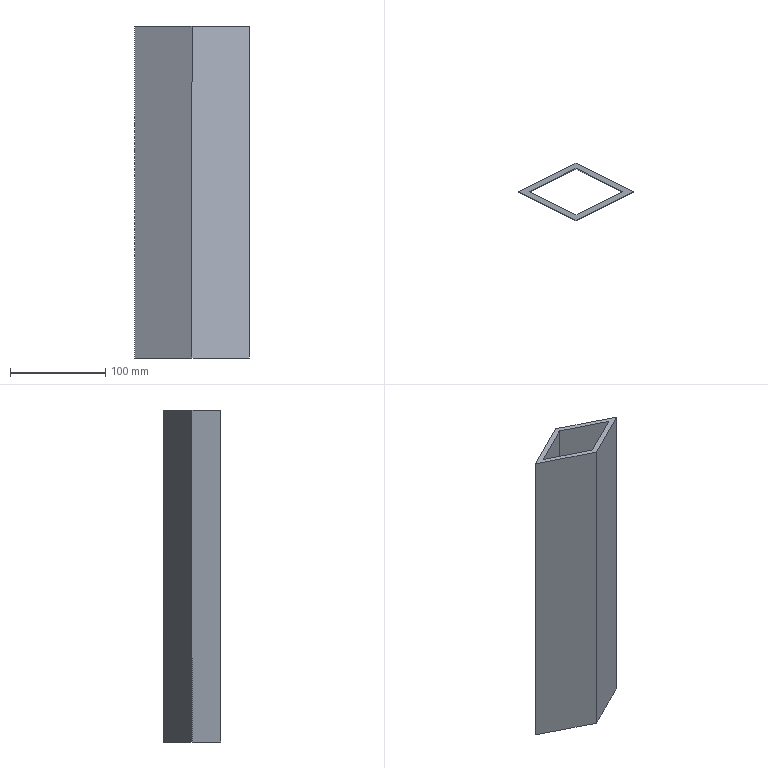Part | SolidWorks | features Cut 1, Extrusion 1 | 1 solid | 10 faces | box 120 x 60 x 348 mm | volume 423391 mm3 | plane 10
STEP:
#1=CARTESIAN_POINT('',(60.,139.912,0.));
#2=VERTEX_POINT('',#1);
#3=CARTESIAN_POINT('',(0.,169.912,0.));
#4=VERTEX_POINT('',#3);
#5=CARTESIAN_POINT('',(60.,139.912,0.));
#6=DIRECTION('',(-0.8944,0.4472,0.));
#7=VECTOR('',#6,1000.);
#8=LINE('',#5,#7);
#9=EDGE_CURVE('',#2,#4,#8,.T.);
#10=ORIENTED_EDGE('',*,*,#9,.T.);
#11=CARTESIAN_POINT('',(0.,169.912,348.));
#12=VERTEX_POINT('',#11);
#13=CARTESIAN_POINT('',(0.,169.912,348.));
#14=DIRECTION('',(0.,0.,-1.));
#15=VECTOR('',#14,1000.);
#16=LINE('',#13,#15);
#17=EDGE_CURVE('',#12,#4,#16,.T.);
#18=ORIENTED_EDGE('',*,*,#17,.F.);
#19=CARTESIAN_POINT('',(60.,139.912,348.));
#20=VERTEX_POINT('',#19);
#21=CARTESIAN_POINT('',(60.,139.912,348.));
#22=DIRECTION('',(-0.8944,0.4472,0.));
#23=VECTOR('',#22,1000.);
#24=LINE('',#21,#23);
#25=EDGE_CURVE('',#20,#12,#24,.T.);
#26=ORIENTED_EDGE('',*,*,#25,.F.);
#27=CARTESIAN_POINT('',(60.,139.912,348.));
#28=DIRECTION('',(0.,0.,-1.));
#29=VECTOR('',#28,1000.);
#30=LINE('',#27,#29);
#31=EDGE_CURVE('',#20,#2,#30,.T.);
#32=ORIENTED_EDGE('',*,*,#31,.T.);
#33=EDGE_LOOP('',(#10,#18,#26,#32));
#34=FACE_OUTER_BOUND('',#33,.T.);
#35=CARTESIAN_POINT('',(60.,139.912,348.));
#36=DIRECTION('',(-0.4472,-0.8944,0.));
#37=DIRECTION('',(0.8944,-0.4472,0.));
#38=AXIS2_PLACEMENT_3D('',#35,#36,#37);
#39=PLANE('',#38);
#40=ADVANCED_FACE('',(#34),#39,.F.);
#41=CARTESIAN_POINT('',(-60.,139.912,0.));
#42=VERTEX_POINT('',#41);
#43=CARTESIAN_POINT('',(0.,169.912,0.));
#44=DIRECTION('',(-0.8944,-0.4472,0.));
#45=VECTOR('',#44,1000.);
#46=LINE('',#43,#45);
#47=EDGE_CURVE('',#4,#42,#46,.T.);
#48=ORIENTED_EDGE('',*,*,#47,.T.);
#49=CARTESIAN_POINT('',(-60.,139.912,348.));
#50=VERTEX_POINT('',#49);
#51=CARTESIAN_POINT('',(-60.,139.912,348.));
#52=DIRECTION('',(0.,0.,-1.));
#53=VECTOR('',#52,1000.);
#54=LINE('',#51,#53);
#55=EDGE_CURVE('',#50,#42,#54,.T.);
#56=ORIENTED_EDGE('',*,*,#55,.F.);
#57=CARTESIAN_POINT('',(0.,169.912,348.));
#58=DIRECTION('',(-0.8944,-0.4472,0.));
#59=VECTOR('',#58,1000.);
#60=LINE('',#57,#59);
#61=EDGE_CURVE('',#12,#50,#60,.T.);
#62=ORIENTED_EDGE('',*,*,#61,.F.);
#63=ORIENTED_EDGE('',*,*,#17,.T.);
#64=EDGE_LOOP('',(#48,#56,#62,#63));
#65=FACE_OUTER_BOUND('',#64,.T.);
#66=CARTESIAN_POINT('',(0.,169.912,348.));
#67=DIRECTION('',(0.4472,-0.8944,0.));
#68=DIRECTION('',(0.8944,0.4472,0.));
#69=AXIS2_PLACEMENT_3D('',#66,#67,#68);
#70=PLANE('',#69);
#71=ADVANCED_FACE('',(#65),#70,.F.);
#72=CARTESIAN_POINT('',(0.,109.912,0.));
#73=VERTEX_POINT('',#72);
#74=CARTESIAN_POINT('',(-60.,139.912,0.));
#75=DIRECTION('',(0.8944,-0.4472,0.));
#76=VECTOR('',#75,1000.);
#77=LINE('',#74,#76);
#78=EDGE_CURVE('',#42,#73,#77,.T.);
#79=ORIENTED_EDGE('',*,*,#78,.T.);
#80=CARTESIAN_POINT('',(0.,109.912,348.));
#81=VERTEX_POINT('',#80);
#82=CARTESIAN_POINT('',(0.,109.912,348.));
#83=DIRECTION('',(0.,0.,-1.));
#84=VECTOR('',#83,1000.);
#85=LINE('',#82,#84);
#86=EDGE_CURVE('',#81,#73,#85,.T.);
#87=ORIENTED_EDGE('',*,*,#86,.F.);
#88=CARTESIAN_POINT('',(-60.,139.912,348.));
#89=DIRECTION('',(0.8944,-0.4472,0.));
#90=VECTOR('',#89,1000.);
#91=LINE('',#88,#90);
#92=EDGE_CURVE('',#50,#81,#91,.T.);
#93=ORIENTED_EDGE('',*,*,#92,.F.);
#94=ORIENTED_EDGE('',*,*,#55,.T.);
#95=EDGE_LOOP('',(#79,#87,#93,#94));
#96=FACE_OUTER_BOUND('',#95,.T.);
#97=CARTESIAN_POINT('',(-60.,139.912,348.));
#98=DIRECTION('',(0.4472,0.8944,0.));
#99=DIRECTION('',(-0.8944,0.4472,0.));
#100=AXIS2_PLACEMENT_3D('',#97,#98,#99);
#101=PLANE('',#100);
#102=ADVANCED_FACE('',(#96),#101,.F.);
#103=CARTESIAN_POINT('',(0.,109.912,0.));
#104=DIRECTION('',(0.8944,0.4472,0.));
#105=VECTOR('',#104,1000.);
#106=LINE('',#103,#105);
#107=EDGE_CURVE('',#73,#2,#106,.T.);
#108=ORIENTED_EDGE('',*,*,#107,.T.);
#109=ORIENTED_EDGE('',*,*,#31,.F.);
#110=CARTESIAN_POINT('',(0.,109.912,348.));
#111=DIRECTION('',(0.8944,0.4472,0.));
#112=VECTOR('',#111,1000.);
#113=LINE('',#110,#112);
#114=EDGE_CURVE('',#81,#20,#113,.T.);
#115=ORIENTED_EDGE('',*,*,#114,.F.);
#116=ORIENTED_EDGE('',*,*,#86,.T.);
#117=EDGE_LOOP('',(#108,#109,#115,#116));
#118=FACE_OUTER_BOUND('',#117,.T.);
#119=CARTESIAN_POINT('',(0.,109.912,348.));
#120=DIRECTION('',(-0.4472,0.8944,0.));
#121=DIRECTION('',(-0.8944,-0.4472,0.));
#122=AXIS2_PLACEMENT_3D('',#119,#120,#121);
#123=PLANE('',#122);
#124=ADVANCED_FACE('',(#118),#123,.F.);
#125=CARTESIAN_POINT('',(0.,115.502,348.));
#126=VERTEX_POINT('',#125);
#127=CARTESIAN_POINT('',(48.82,139.912,348.));
#128=VERTEX_POINT('',#127);
#129=CARTESIAN_POINT('',(0.,115.502,348.));
#130=DIRECTION('',(0.8944,0.4472,0.));
#131=VECTOR('',#130,1000.);
#132=LINE('',#129,#131);
#133=EDGE_CURVE('',#126,#128,#132,.T.);
#134=ORIENTED_EDGE('',*,*,#133,.F.);
#135=CARTESIAN_POINT('',(-48.82,139.912,348.));
#136=VERTEX_POINT('',#135);
#137=CARTESIAN_POINT('',(-48.82,139.912,348.));
#138=DIRECTION('',(0.8944,-0.4472,0.));
#139=VECTOR('',#138,1000.);
#140=LINE('',#137,#139);
#141=EDGE_CURVE('',#136,#126,#140,.T.);
#142=ORIENTED_EDGE('',*,*,#141,.F.);
#143=CARTESIAN_POINT('',(0.,164.321,348.));
#144=VERTEX_POINT('',#143);
#145=CARTESIAN_POINT('',(0.,164.321,348.));
#146=DIRECTION('',(-0.8944,-0.4472,0.));
#147=VECTOR('',#146,1000.);
#148=LINE('',#145,#147);
#149=EDGE_CURVE('',#144,#136,#148,.T.);
#150=ORIENTED_EDGE('',*,*,#149,.F.);
#151=CARTESIAN_POINT('',(48.82,139.912,348.));
#152=DIRECTION('',(-0.8944,0.4472,0.));
#153=VECTOR('',#152,1000.);
#154=LINE('',#151,#153);
#155=EDGE_CURVE('',#128,#144,#154,.T.);
#156=ORIENTED_EDGE('',*,*,#155,.F.);
#157=EDGE_LOOP('',(#134,#142,#150,#156));
#158=FACE_BOUND('',#157,.T.);
#159=ORIENTED_EDGE('',*,*,#25,.T.);
#160=ORIENTED_EDGE('',*,*,#61,.T.);
#161=ORIENTED_EDGE('',*,*,#92,.T.);
#162=ORIENTED_EDGE('',*,*,#114,.T.);
#163=EDGE_LOOP('',(#159,#160,#161,#162));
#164=FACE_OUTER_BOUND('',#163,.T.);
#165=CARTESIAN_POINT('',(0.,0.,348.));
#166=DIRECTION('',(0.,0.,1.));
#167=DIRECTION('',(1.,0.,0.));
#168=AXIS2_PLACEMENT_3D('',#165,#166,#167);
#169=PLANE('',#168);
#170=ADVANCED_FACE('',(#158,#164),#169,.T.);
#171=CARTESIAN_POINT('',(-48.82,139.912,0.));
#172=VERTEX_POINT('',#171);
#173=CARTESIAN_POINT('',(0.,115.502,0.));
#174=VERTEX_POINT('',#173);
#175=CARTESIAN_POINT('',(46.201,92.401,0.));
#176=DIRECTION('',(0.8944,-0.4472,0.));
#177=VECTOR('',#176,1000.);
#178=LINE('',#175,#177);
#179=EDGE_CURVE('',#172,#174,#178,.T.);
#180=ORIENTED_EDGE('',*,*,#179,.T.);
#181=CARTESIAN_POINT('',(48.82,139.912,0.));
#182=VERTEX_POINT('',#181);
#183=CARTESIAN_POINT('',(-46.201,92.401,0.));
#184=DIRECTION('',(0.8944,0.4472,0.));
#185=VECTOR('',#184,1000.);
#186=LINE('',#183,#185);
#187=EDGE_CURVE('',#174,#182,#186,.T.);
#188=ORIENTED_EDGE('',*,*,#187,.T.);
#189=CARTESIAN_POINT('',(0.,164.321,0.));
#190=VERTEX_POINT('',#189);
#191=CARTESIAN_POINT('',(65.729,131.457,0.));
#192=DIRECTION('',(-0.8944,0.4472,0.));
#193=VECTOR('',#192,1000.);
#194=LINE('',#191,#193);
#195=EDGE_CURVE('',#182,#190,#194,.T.);
#196=ORIENTED_EDGE('',*,*,#195,.T.);
#197=CARTESIAN_POINT('',(-65.729,131.457,0.));
#198=DIRECTION('',(-0.8944,-0.4472,0.));
#199=VECTOR('',#198,1000.);
#200=LINE('',#197,#199);
#201=EDGE_CURVE('',#190,#172,#200,.T.);
#202=ORIENTED_EDGE('',*,*,#201,.T.);
#203=EDGE_LOOP('',(#180,#188,#196,#202));
#204=FACE_BOUND('',#203,.T.);
#205=ORIENTED_EDGE('',*,*,#9,.F.);
#206=ORIENTED_EDGE('',*,*,#107,.F.);
#207=ORIENTED_EDGE('',*,*,#78,.F.);
#208=ORIENTED_EDGE('',*,*,#47,.F.);
#209=EDGE_LOOP('',(#205,#206,#207,#208));
#210=FACE_OUTER_BOUND('',#209,.T.);
#211=CARTESIAN_POINT('',(0.,0.,0.));
#212=DIRECTION('',(0.,0.,1.));
#213=DIRECTION('',(1.,0.,0.));
#214=AXIS2_PLACEMENT_3D('',#211,#212,#213);
#215=PLANE('',#214);
#216=ADVANCED_FACE('',(#204,#210),#215,.F.);
#217=CARTESIAN_POINT('',(0.,115.502,-2.));
#218=DIRECTION('',(0.,0.,1.));
#219=VECTOR('',#218,1000.);
#220=LINE('',#217,#219);
#221=EDGE_CURVE('',#174,#126,#220,.T.);
#222=ORIENTED_EDGE('',*,*,#221,.T.);
#223=ORIENTED_EDGE('',*,*,#133,.T.);
#224=CARTESIAN_POINT('',(48.82,139.912,-2.));
#225=DIRECTION('',(0.,0.,1.));
#226=VECTOR('',#225,1000.);
#227=LINE('',#224,#226);
#228=EDGE_CURVE('',#182,#128,#227,.T.);
#229=ORIENTED_EDGE('',*,*,#228,.F.);
#230=ORIENTED_EDGE('',*,*,#187,.F.);
#231=EDGE_LOOP('',(#222,#223,#229,#230));
#232=FACE_OUTER_BOUND('',#231,.T.);
#233=CARTESIAN_POINT('',(0.,115.502,-2.));
#234=DIRECTION('',(0.4472,-0.8944,0.));
#235=DIRECTION('',(0.8944,0.4472,0.));
#236=AXIS2_PLACEMENT_3D('',#233,#234,#235);
#237=PLANE('',#236);
#238=ADVANCED_FACE('',(#232),#237,.F.);
#239=CARTESIAN_POINT('',(-48.82,139.912,-2.));
#240=DIRECTION('',(0.,0.,1.));
#241=VECTOR('',#240,1000.);
#242=LINE('',#239,#241);
#243=EDGE_CURVE('',#172,#136,#242,.T.);
#244=ORIENTED_EDGE('',*,*,#243,.T.);
#245=ORIENTED_EDGE('',*,*,#141,.T.);
#246=ORIENTED_EDGE('',*,*,#221,.F.);
#247=ORIENTED_EDGE('',*,*,#179,.F.);
#248=EDGE_LOOP('',(#244,#245,#246,#247));
#249=FACE_OUTER_BOUND('',#248,.T.);
#250=CARTESIAN_POINT('',(-48.82,139.912,-2.));
#251=DIRECTION('',(-0.4472,-0.8944,0.));
#252=DIRECTION('',(0.8944,-0.4472,0.));
#253=AXIS2_PLACEMENT_3D('',#250,#251,#252);
#254=PLANE('',#253);
#255=ADVANCED_FACE('',(#249),#254,.F.);
#256=CARTESIAN_POINT('',(0.,164.321,-2.));
#257=DIRECTION('',(0.,0.,1.));
#258=VECTOR('',#257,1000.);
#259=LINE('',#256,#258);
#260=EDGE_CURVE('',#190,#144,#259,.T.);
#261=ORIENTED_EDGE('',*,*,#260,.T.);
#262=ORIENTED_EDGE('',*,*,#149,.T.);
#263=ORIENTED_EDGE('',*,*,#243,.F.);
#264=ORIENTED_EDGE('',*,*,#201,.F.);
#265=EDGE_LOOP('',(#261,#262,#263,#264));
#266=FACE_OUTER_BOUND('',#265,.T.);
#267=CARTESIAN_POINT('',(0.,164.321,-2.));
#268=DIRECTION('',(-0.4472,0.8944,0.));
#269=DIRECTION('',(-0.8944,-0.4472,0.));
#270=AXIS2_PLACEMENT_3D('',#267,#268,#269);
#271=PLANE('',#270);
#272=ADVANCED_FACE('',(#266),#271,.F.);
#273=ORIENTED_EDGE('',*,*,#228,.T.);
#274=ORIENTED_EDGE('',*,*,#155,.T.);
#275=ORIENTED_EDGE('',*,*,#260,.F.);
#276=ORIENTED_EDGE('',*,*,#195,.F.);
#277=EDGE_LOOP('',(#273,#274,#275,#276));
#278=FACE_OUTER_BOUND('',#277,.T.);
#279=CARTESIAN_POINT('',(48.82,139.912,-2.));
#280=DIRECTION('',(0.4472,0.8944,0.));
#281=DIRECTION('',(-0.8944,0.4472,0.));
#282=AXIS2_PLACEMENT_3D('',#279,#280,#281);
#283=PLANE('',#282);
#284=ADVANCED_FACE('',(#278),#283,.F.);
#285=CLOSED_SHELL('',(#40,#71,#102,#124,#170,#216,#238,#255,#272,#284));
#286=MANIFOLD_SOLID_BREP('',#285);
#287=CARTESIAN_POINT('',(0.,0.,0.));
#288=DIRECTION('',(0.,0.,1.));
#289=DIRECTION('',(1.,0.,0.));
#290=AXIS2_PLACEMENT_3D('',#287,#288,#289);
#291=(LENGTH_UNIT()NAMED_UNIT(*)SI_UNIT(.MILLI.,.METRE.));
#292=UNCERTAINTY_MEASURE_WITH_UNIT(LENGTH_MEASURE(0.00001),#291,'','');
#293=(NAMED_UNIT(*)PLANE_ANGLE_UNIT()SI_UNIT($,.RADIAN.));
#294=(NAMED_UNIT(*)SI_UNIT($,.STERADIAN.)SOLID_ANGLE_UNIT());
#295=(GEOMETRIC_REPRESENTATION_CONTEXT(3)GLOBAL_UNCERTAINTY_ASSIGNED_CONTEXT((#292))GLOBAL_UNIT_ASSIGNED_CONTEXT((#291,#293,#294))REPRESENTATION_CONTEXT('',''));
#296=ADVANCED_BREP_SHAPE_REPRESENTATION('',(#286,#290),#295);